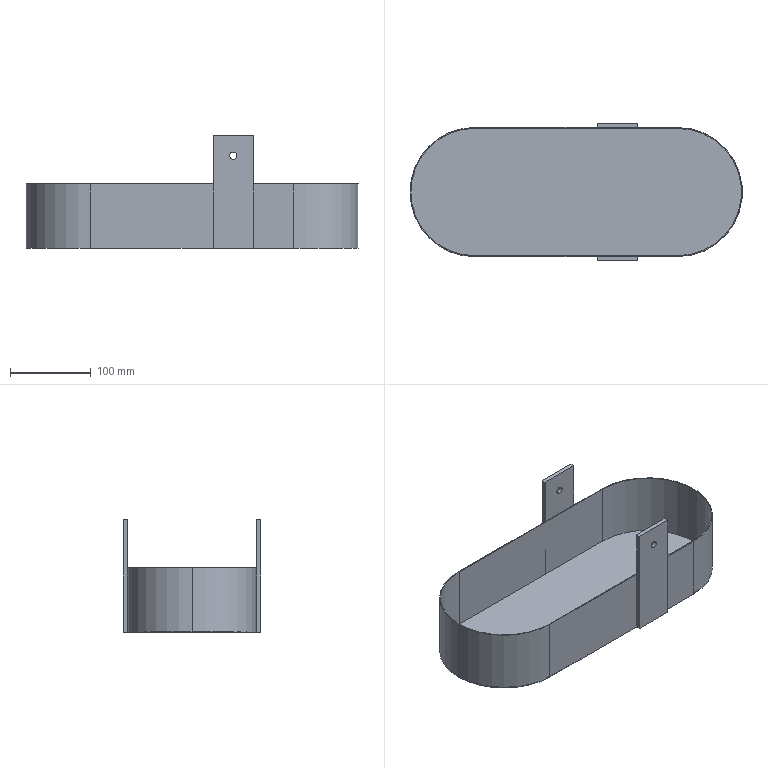Part | STEP file | Guard cover 2 | 1 solid | 29 faces | box 412.05 x 170 x 140 mm | volume 209083 mm3 | plane 19 | cylinder 10 | commonest cylinder face diameters 9 x4 158 x3 160 x3